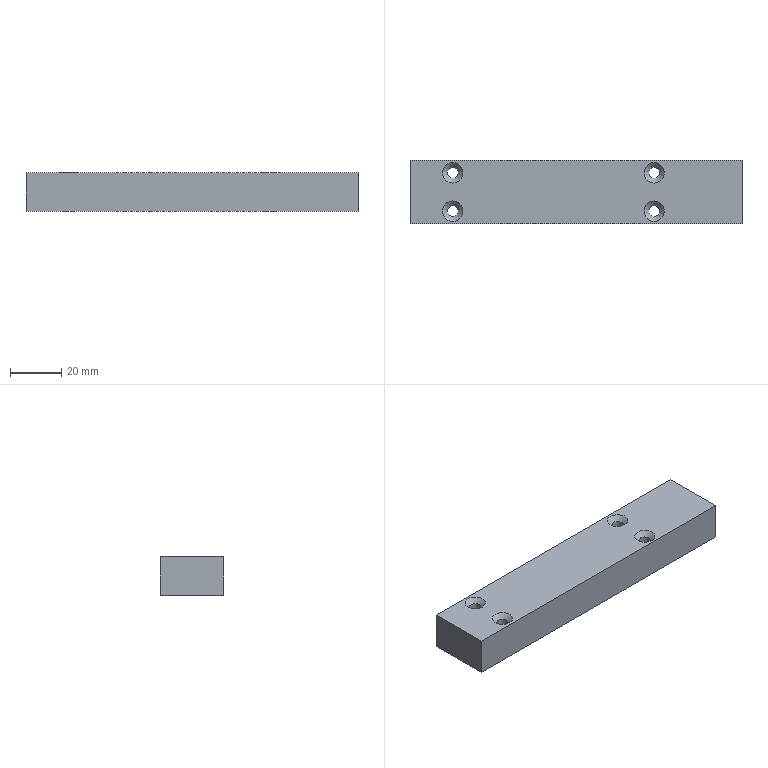Part | STEP file | Chassis spacer strip 2 | 1 solid | 24 faces | box 130 x 25 x 15 mm | volume 47613 mm3 | cone 12 | plane 6 | cylinder 6 | commonest cylinder face diameters 4.3 x4 3.3 x2